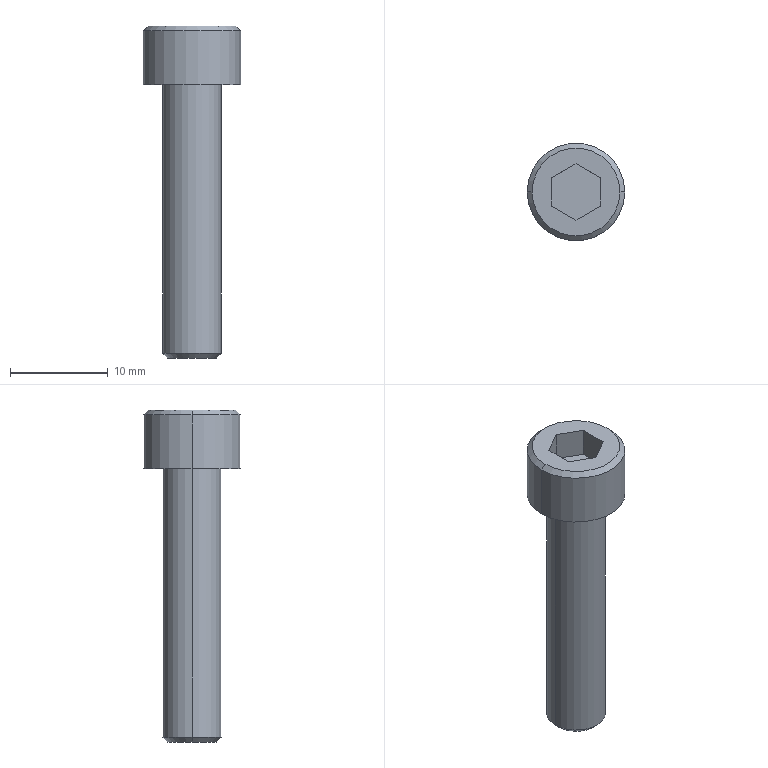Part | Creo | 1 solid | 18 faces | box 10 x 10 x 34 mm | volume 1192 mm3 | plane 10 | cone 4 | cylinder 4 | commonest cylinder face diameters 6 x2 10 x2
STEP:
#1=CARTESIAN_POINT('',(4.5,135.,-211.5));
#2=VERTEX_POINT('',#1);
#3=CARTESIAN_POINT('',(-4.5,135.,-211.5));
#4=VERTEX_POINT('',#3);
#5=CARTESIAN_POINT('',(0.,135.,-211.5));
#6=DIRECTION('',(0.,0.,1.));
#7=DIRECTION('',(1.,0.,0.));
#8=AXIS2_PLACEMENT_3D('',#5,#6,#7);
#9=CIRCLE('',#8,4.5);
#10=EDGE_CURVE('',#2,#4,#9,.T.);
#11=ORIENTED_EDGE('',*,*,#10,.F.);
#12=CARTESIAN_POINT('',(0.,135.,-211.5));
#13=DIRECTION('',(0.,0.,1.));
#14=DIRECTION('',(-1.,0.,0.));
#15=AXIS2_PLACEMENT_3D('',#12,#13,#14);
#16=CIRCLE('',#15,4.5);
#17=EDGE_CURVE('',#4,#2,#16,.T.);
#18=ORIENTED_EDGE('',*,*,#17,.F.);
#19=EDGE_LOOP('',(#11,#18));
#20=FACE_OUTER_BOUND('',#19,.F.);
#21=CARTESIAN_POINT('',(-2.5,133.557,-211.5));
#22=VERTEX_POINT('',#21);
#23=CARTESIAN_POINT('',(-2.5,136.443,-211.5));
#24=VERTEX_POINT('',#23);
#25=CARTESIAN_POINT('',(-2.5,133.557,-211.5));
#26=DIRECTION('',(0.,1.,0.));
#27=VECTOR('',#26,2.887);
#28=LINE('',#25,#27);
#29=EDGE_CURVE('',#22,#24,#28,.T.);
#30=ORIENTED_EDGE('',*,*,#29,.F.);
#31=CARTESIAN_POINT('',(0.,132.113,-211.5));
#32=VERTEX_POINT('',#31);
#33=CARTESIAN_POINT('',(0.,132.113,-211.5));
#34=DIRECTION('',(-0.866,0.5,0.));
#35=VECTOR('',#34,2.887);
#36=LINE('',#33,#35);
#37=EDGE_CURVE('',#32,#22,#36,.T.);
#38=ORIENTED_EDGE('',*,*,#37,.F.);
#39=CARTESIAN_POINT('',(2.5,133.557,-211.5));
#40=VERTEX_POINT('',#39);
#41=CARTESIAN_POINT('',(2.5,133.557,-211.5));
#42=DIRECTION('',(-0.866,-0.5,0.));
#43=VECTOR('',#42,2.887);
#44=LINE('',#41,#43);
#45=EDGE_CURVE('',#40,#32,#44,.T.);
#46=ORIENTED_EDGE('',*,*,#45,.F.);
#47=CARTESIAN_POINT('',(2.5,136.443,-211.5));
#48=VERTEX_POINT('',#47);
#49=CARTESIAN_POINT('',(2.5,136.443,-211.5));
#50=DIRECTION('',(0.,-1.,0.));
#51=VECTOR('',#50,2.887);
#52=LINE('',#49,#51);
#53=EDGE_CURVE('',#48,#40,#52,.T.);
#54=ORIENTED_EDGE('',*,*,#53,.F.);
#55=CARTESIAN_POINT('',(0.,137.887,-211.5));
#56=VERTEX_POINT('',#55);
#57=CARTESIAN_POINT('',(0.,137.887,-211.5));
#58=DIRECTION('',(0.866,-0.5,0.));
#59=VECTOR('',#58,2.887);
#60=LINE('',#57,#59);
#61=EDGE_CURVE('',#56,#48,#60,.T.);
#62=ORIENTED_EDGE('',*,*,#61,.F.);
#63=CARTESIAN_POINT('',(-2.5,136.443,-211.5));
#64=DIRECTION('',(0.866,0.5,0.));
#65=VECTOR('',#64,2.887);
#66=LINE('',#63,#65);
#67=EDGE_CURVE('',#24,#56,#66,.T.);
#68=ORIENTED_EDGE('',*,*,#67,.F.);
#69=EDGE_LOOP('',(#30,#38,#46,#54,#62,#68));
#70=FACE_BOUND('',#69,.F.);
#71=CARTESIAN_POINT('',(0.,135.,-211.5));
#72=DIRECTION('',(0.,0.,1.));
#73=DIRECTION('',(1.,0.,0.));
#74=AXIS2_PLACEMENT_3D('',#71,#72,#73);
#75=PLANE('',#74);
#76=ADVANCED_FACE('',(#20,#70),#75,.T.);
#77=ORIENTED_EDGE('',*,*,#10,.T.);
#78=CARTESIAN_POINT('',(-5.,135.,-212.));
#79=VERTEX_POINT('',#78);
#80=CARTESIAN_POINT('',(-4.5,135.,-211.5));
#81=DIRECTION('',(-0.7071,0.,-0.7071));
#82=VECTOR('',#81,0.7071);
#83=LINE('',#80,#82);
#84=EDGE_CURVE('',#4,#79,#83,.T.);
#85=ORIENTED_EDGE('',*,*,#84,.T.);
#86=CARTESIAN_POINT('',(5.,135.,-212.));
#87=VERTEX_POINT('',#86);
#88=CARTESIAN_POINT('',(0.,135.,-212.));
#89=DIRECTION('',(0.,0.,1.));
#90=DIRECTION('',(1.,0.,0.));
#91=AXIS2_PLACEMENT_3D('',#88,#89,#90);
#92=CIRCLE('',#91,5.);
#93=EDGE_CURVE('',#87,#79,#92,.T.);
#94=ORIENTED_EDGE('',*,*,#93,.F.);
#95=CARTESIAN_POINT('',(4.5,135.,-211.5));
#96=DIRECTION('',(0.7071,0.,-0.7071));
#97=VECTOR('',#96,0.7071);
#98=LINE('',#95,#97);
#99=EDGE_CURVE('',#2,#87,#98,.T.);
#100=ORIENTED_EDGE('',*,*,#99,.F.);
#101=EDGE_LOOP('',(#77,#85,#94,#100));
#102=FACE_OUTER_BOUND('',#101,.F.);
#103=CARTESIAN_POINT('',(0.,135.,-211.75));
#104=DIRECTION('',(0.,0.,-1.));
#105=DIRECTION('',(-1.,0.,0.));
#106=AXIS2_PLACEMENT_3D('',#103,#104,#105);
#107=CONICAL_SURFACE('',#106,4.75,45.);
#108=ADVANCED_FACE('',(#102),#107,.T.);
#109=ORIENTED_EDGE('',*,*,#17,.T.);
#110=ORIENTED_EDGE('',*,*,#99,.T.);
#111=CARTESIAN_POINT('',(0.,135.,-212.));
#112=DIRECTION('',(0.,0.,1.));
#113=DIRECTION('',(-1.,0.,0.));
#114=AXIS2_PLACEMENT_3D('',#111,#112,#113);
#115=CIRCLE('',#114,5.);
#116=EDGE_CURVE('',#79,#87,#115,.T.);
#117=ORIENTED_EDGE('',*,*,#116,.F.);
#118=ORIENTED_EDGE('',*,*,#84,.F.);
#119=EDGE_LOOP('',(#109,#110,#117,#118));
#120=FACE_OUTER_BOUND('',#119,.F.);
#121=CARTESIAN_POINT('',(0.,135.,-211.75));
#122=DIRECTION('',(0.,0.,-1.));
#123=DIRECTION('',(-1.,0.,0.));
#124=AXIS2_PLACEMENT_3D('',#121,#122,#123);
#125=CONICAL_SURFACE('',#124,4.75,45.);
#126=ADVANCED_FACE('',(#120),#125,.T.);
#127=ORIENTED_EDGE('',*,*,#116,.T.);
#128=CARTESIAN_POINT('',(5.,135.,-217.5));
#129=VERTEX_POINT('',#128);
#130=CARTESIAN_POINT('',(5.,135.,-217.5));
#131=DIRECTION('',(0.,0.,1.));
#132=VECTOR('',#131,5.5);
#133=LINE('',#130,#132);
#134=EDGE_CURVE('',#129,#87,#133,.T.);
#135=ORIENTED_EDGE('',*,*,#134,.F.);
#136=CARTESIAN_POINT('',(-5.,135.,-217.5));
#137=VERTEX_POINT('',#136);
#138=CARTESIAN_POINT('',(0.,135.,-217.5));
#139=DIRECTION('',(0.,0.,-1.));
#140=DIRECTION('',(1.,0.,0.));
#141=AXIS2_PLACEMENT_3D('',#138,#139,#140);
#142=CIRCLE('',#141,5.);
#143=EDGE_CURVE('',#129,#137,#142,.T.);
#144=ORIENTED_EDGE('',*,*,#143,.T.);
#145=CARTESIAN_POINT('',(-5.,135.,-217.5));
#146=DIRECTION('',(0.,0.,1.));
#147=VECTOR('',#146,5.5);
#148=LINE('',#145,#147);
#149=EDGE_CURVE('',#137,#79,#148,.T.);
#150=ORIENTED_EDGE('',*,*,#149,.T.);
#151=EDGE_LOOP('',(#127,#135,#144,#150));
#152=FACE_OUTER_BOUND('',#151,.F.);
#153=CARTESIAN_POINT('',(0.,135.,-217.5));
#154=DIRECTION('',(0.,0.,1.));
#155=DIRECTION('',(1.,0.,0.));
#156=AXIS2_PLACEMENT_3D('',#153,#154,#155);
#157=CYLINDRICAL_SURFACE('',#156,5.);
#158=ADVANCED_FACE('',(#152),#157,.T.);
#159=ORIENTED_EDGE('',*,*,#93,.T.);
#160=ORIENTED_EDGE('',*,*,#149,.F.);
#161=CARTESIAN_POINT('',(0.,135.,-217.5));
#162=DIRECTION('',(0.,0.,-1.));
#163=DIRECTION('',(-1.,0.,0.));
#164=AXIS2_PLACEMENT_3D('',#161,#162,#163);
#165=CIRCLE('',#164,5.);
#166=EDGE_CURVE('',#137,#129,#165,.T.);
#167=ORIENTED_EDGE('',*,*,#166,.T.);
#168=ORIENTED_EDGE('',*,*,#134,.T.);
#169=EDGE_LOOP('',(#159,#160,#167,#168));
#170=FACE_OUTER_BOUND('',#169,.F.);
#171=CARTESIAN_POINT('',(0.,135.,-217.5));
#172=DIRECTION('',(0.,0.,1.));
#173=DIRECTION('',(1.,0.,0.));
#174=AXIS2_PLACEMENT_3D('',#171,#172,#173);
#175=CYLINDRICAL_SURFACE('',#174,5.);
#176=ADVANCED_FACE('',(#170),#175,.T.);
#177=ORIENTED_EDGE('',*,*,#143,.F.);
#178=ORIENTED_EDGE('',*,*,#166,.F.);
#179=EDGE_LOOP('',(#177,#178));
#180=FACE_OUTER_BOUND('',#179,.F.);
#181=CARTESIAN_POINT('',(-3.,135.,-217.5));
#182=VERTEX_POINT('',#181);
#183=CARTESIAN_POINT('',(3.,135.,-217.5));
#184=VERTEX_POINT('',#183);
#185=CARTESIAN_POINT('',(0.,135.,-217.5));
#186=DIRECTION('',(0.,0.,1.));
#187=DIRECTION('',(-1.,0.,0.));
#188=AXIS2_PLACEMENT_3D('',#185,#186,#187);
#189=CIRCLE('',#188,3.);
#190=EDGE_CURVE('',#182,#184,#189,.T.);
#191=ORIENTED_EDGE('',*,*,#190,.F.);
#192=CARTESIAN_POINT('',(0.,135.,-217.5));
#193=DIRECTION('',(0.,0.,1.));
#194=DIRECTION('',(1.,0.,0.));
#195=AXIS2_PLACEMENT_3D('',#192,#193,#194);
#196=CIRCLE('',#195,3.);
#197=EDGE_CURVE('',#184,#182,#196,.T.);
#198=ORIENTED_EDGE('',*,*,#197,.F.);
#199=EDGE_LOOP('',(#191,#198));
#200=FACE_BOUND('',#199,.F.);
#201=CARTESIAN_POINT('',(0.,135.,-217.5));
#202=DIRECTION('',(0.,0.,-1.));
#203=DIRECTION('',(-1.,0.,0.));
#204=AXIS2_PLACEMENT_3D('',#201,#202,#203);
#205=PLANE('',#204);
#206=ADVANCED_FACE('',(#180,#200),#205,.T.);
#207=CARTESIAN_POINT('',(3.,135.,-245.));
#208=VERTEX_POINT('',#207);
#209=CARTESIAN_POINT('',(-3.,135.,-245.));
#210=VERTEX_POINT('',#209);
#211=CARTESIAN_POINT('',(0.,135.,-245.));
#212=DIRECTION('',(0.,0.,-1.));
#213=DIRECTION('',(1.,0.,0.));
#214=AXIS2_PLACEMENT_3D('',#211,#212,#213);
#215=CIRCLE('',#214,3.);
#216=EDGE_CURVE('',#208,#210,#215,.T.);
#217=ORIENTED_EDGE('',*,*,#216,.T.);
#218=CARTESIAN_POINT('',(-3.,135.,-217.5));
#219=DIRECTION('',(0.,0.,-1.));
#220=VECTOR('',#219,27.5);
#221=LINE('',#218,#220);
#222=EDGE_CURVE('',#182,#210,#221,.T.);
#223=ORIENTED_EDGE('',*,*,#222,.F.);
#224=ORIENTED_EDGE('',*,*,#190,.T.);
#225=CARTESIAN_POINT('',(3.,135.,-217.5));
#226=DIRECTION('',(0.,0.,-1.));
#227=VECTOR('',#226,27.5);
#228=LINE('',#225,#227);
#229=EDGE_CURVE('',#184,#208,#228,.T.);
#230=ORIENTED_EDGE('',*,*,#229,.T.);
#231=EDGE_LOOP('',(#217,#223,#224,#230));
#232=FACE_OUTER_BOUND('',#231,.F.);
#233=CARTESIAN_POINT('',(0.,135.,-217.5));
#234=DIRECTION('',(0.,0.,-1.));
#235=DIRECTION('',(-1.,0.,0.));
#236=AXIS2_PLACEMENT_3D('',#233,#234,#235);
#237=CYLINDRICAL_SURFACE('',#236,3.);
#238=ADVANCED_FACE('',(#232),#237,.T.);
#239=CARTESIAN_POINT('',(2.5,135.,-245.5));
#240=VERTEX_POINT('',#239);
#241=CARTESIAN_POINT('',(-2.5,135.,-245.5));
#242=VERTEX_POINT('',#241);
#243=CARTESIAN_POINT('',(0.,135.,-245.5));
#244=DIRECTION('',(0.,0.,-1.));
#245=DIRECTION('',(1.,0.,0.));
#246=AXIS2_PLACEMENT_3D('',#243,#244,#245);
#247=CIRCLE('',#246,2.5);
#248=EDGE_CURVE('',#240,#242,#247,.T.);
#249=ORIENTED_EDGE('',*,*,#248,.T.);
#250=CARTESIAN_POINT('',(-2.5,135.,-245.5));
#251=DIRECTION('',(-0.7071,0.,0.7071));
#252=VECTOR('',#251,0.7071);
#253=LINE('',#250,#252);
#254=EDGE_CURVE('',#242,#210,#253,.T.);
#255=ORIENTED_EDGE('',*,*,#254,.T.);
#256=ORIENTED_EDGE('',*,*,#216,.F.);
#257=CARTESIAN_POINT('',(2.5,135.,-245.5));
#258=DIRECTION('',(0.7071,0.,0.7071));
#259=VECTOR('',#258,0.7071);
#260=LINE('',#257,#259);
#261=EDGE_CURVE('',#240,#208,#260,.T.);
#262=ORIENTED_EDGE('',*,*,#261,.F.);
#263=EDGE_LOOP('',(#249,#255,#256,#262));
#264=FACE_OUTER_BOUND('',#263,.F.);
#265=CARTESIAN_POINT('',(0.,135.,-245.25));
#266=DIRECTION('',(0.,0.,1.));
#267=DIRECTION('',(1.,0.,0.));
#268=AXIS2_PLACEMENT_3D('',#265,#266,#267);
#269=CONICAL_SURFACE('',#268,2.75,45.);
#270=ADVANCED_FACE('',(#264),#269,.T.);
#271=CARTESIAN_POINT('',(0.,135.,-245.5));
#272=DIRECTION('',(0.,0.,-1.));
#273=DIRECTION('',(-1.,0.,0.));
#274=AXIS2_PLACEMENT_3D('',#271,#272,#273);
#275=CIRCLE('',#274,2.5);
#276=EDGE_CURVE('',#242,#240,#275,.T.);
#277=ORIENTED_EDGE('',*,*,#276,.F.);
#278=ORIENTED_EDGE('',*,*,#248,.F.);
#279=EDGE_LOOP('',(#277,#278));
#280=FACE_OUTER_BOUND('',#279,.F.);
#281=CARTESIAN_POINT('',(0.,135.,-245.5));
#282=DIRECTION('',(0.,0.,-1.));
#283=DIRECTION('',(-1.,0.,0.));
#284=AXIS2_PLACEMENT_3D('',#281,#282,#283);
#285=PLANE('',#284);
#286=ADVANCED_FACE('',(#280),#285,.T.);
#287=ORIENTED_EDGE('',*,*,#276,.T.);
#288=ORIENTED_EDGE('',*,*,#261,.T.);
#289=CARTESIAN_POINT('',(0.,135.,-245.));
#290=DIRECTION('',(0.,0.,-1.));
#291=DIRECTION('',(-1.,0.,0.));
#292=AXIS2_PLACEMENT_3D('',#289,#290,#291);
#293=CIRCLE('',#292,3.);
#294=EDGE_CURVE('',#210,#208,#293,.T.);
#295=ORIENTED_EDGE('',*,*,#294,.F.);
#296=ORIENTED_EDGE('',*,*,#254,.F.);
#297=EDGE_LOOP('',(#287,#288,#295,#296));
#298=FACE_OUTER_BOUND('',#297,.F.);
#299=CARTESIAN_POINT('',(0.,135.,-245.25));
#300=DIRECTION('',(0.,0.,1.));
#301=DIRECTION('',(1.,0.,0.));
#302=AXIS2_PLACEMENT_3D('',#299,#300,#301);
#303=CONICAL_SURFACE('',#302,2.75,45.);
#304=ADVANCED_FACE('',(#298),#303,.T.);
#305=ORIENTED_EDGE('',*,*,#294,.T.);
#306=ORIENTED_EDGE('',*,*,#229,.F.);
#307=ORIENTED_EDGE('',*,*,#197,.T.);
#308=ORIENTED_EDGE('',*,*,#222,.T.);
#309=EDGE_LOOP('',(#305,#306,#307,#308));
#310=FACE_OUTER_BOUND('',#309,.F.);
#311=CARTESIAN_POINT('',(0.,135.,-217.5));
#312=DIRECTION('',(0.,0.,-1.));
#313=DIRECTION('',(-1.,0.,0.));
#314=AXIS2_PLACEMENT_3D('',#311,#312,#313);
#315=CYLINDRICAL_SURFACE('',#314,3.);
#316=ADVANCED_FACE('',(#310),#315,.T.);
#317=ORIENTED_EDGE('',*,*,#29,.T.);
#318=CARTESIAN_POINT('',(-2.5,136.443,-214.5));
#319=VERTEX_POINT('',#318);
#320=CARTESIAN_POINT('',(-2.5,136.443,-211.5));
#321=DIRECTION('',(0.,0.,-1.));
#322=VECTOR('',#321,3.);
#323=LINE('',#320,#322);
#324=EDGE_CURVE('',#24,#319,#323,.T.);
#325=ORIENTED_EDGE('',*,*,#324,.T.);
#326=CARTESIAN_POINT('',(-2.5,133.557,-214.5));
#327=VERTEX_POINT('',#326);
#328=CARTESIAN_POINT('',(-2.5,133.557,-214.5));
#329=DIRECTION('',(0.,1.,0.));
#330=VECTOR('',#329,2.887);
#331=LINE('',#328,#330);
#332=EDGE_CURVE('',#327,#319,#331,.T.);
#333=ORIENTED_EDGE('',*,*,#332,.F.);
#334=CARTESIAN_POINT('',(-2.5,133.557,-211.5));
#335=DIRECTION('',(0.,0.,-1.));
#336=VECTOR('',#335,3.);
#337=LINE('',#334,#336);
#338=EDGE_CURVE('',#22,#327,#337,.T.);
#339=ORIENTED_EDGE('',*,*,#338,.F.);
#340=EDGE_LOOP('',(#317,#325,#333,#339));
#341=FACE_OUTER_BOUND('',#340,.F.);
#342=CARTESIAN_POINT('',(-2.5,135.,-213.));
#343=DIRECTION('',(-1.,0.,0.));
#344=DIRECTION('',(0.,0.,1.));
#345=AXIS2_PLACEMENT_3D('',#342,#343,#344);
#346=PLANE('',#345);
#347=ADVANCED_FACE('',(#341),#346,.F.);
#348=ORIENTED_EDGE('',*,*,#67,.T.);
#349=CARTESIAN_POINT('',(0.,137.887,-214.5));
#350=VERTEX_POINT('',#349);
#351=CARTESIAN_POINT('',(0.,137.887,-211.5));
#352=DIRECTION('',(0.,0.,-1.));
#353=VECTOR('',#352,3.);
#354=LINE('',#351,#353);
#355=EDGE_CURVE('',#56,#350,#354,.T.);
#356=ORIENTED_EDGE('',*,*,#355,.T.);
#357=CARTESIAN_POINT('',(0.,137.887,-214.5));
#358=DIRECTION('',(-0.866,-0.5,0.));
#359=VECTOR('',#358,2.887);
#360=LINE('',#357,#359);
#361=EDGE_CURVE('',#350,#319,#360,.T.);
#362=ORIENTED_EDGE('',*,*,#361,.T.);
#363=ORIENTED_EDGE('',*,*,#324,.F.);
#364=EDGE_LOOP('',(#348,#356,#362,#363));
#365=FACE_OUTER_BOUND('',#364,.F.);
#366=CARTESIAN_POINT('',(-1.25,137.165,-213.));
#367=DIRECTION('',(-0.5,0.866,0.));
#368=DIRECTION('',(-0.866,-0.5,0.));
#369=AXIS2_PLACEMENT_3D('',#366,#367,#368);
#370=PLANE('',#369);
#371=ADVANCED_FACE('',(#365),#370,.F.);
#372=ORIENTED_EDGE('',*,*,#61,.T.);
#373=CARTESIAN_POINT('',(2.5,136.443,-214.5));
#374=VERTEX_POINT('',#373);
#375=CARTESIAN_POINT('',(2.5,136.443,-211.5));
#376=DIRECTION('',(0.,0.,-1.));
#377=VECTOR('',#376,3.);
#378=LINE('',#375,#377);
#379=EDGE_CURVE('',#48,#374,#378,.T.);
#380=ORIENTED_EDGE('',*,*,#379,.T.);
#381=CARTESIAN_POINT('',(2.5,136.443,-214.5));
#382=DIRECTION('',(-0.866,0.5,0.));
#383=VECTOR('',#382,2.887);
#384=LINE('',#381,#383);
#385=EDGE_CURVE('',#374,#350,#384,.T.);
#386=ORIENTED_EDGE('',*,*,#385,.T.);
#387=ORIENTED_EDGE('',*,*,#355,.F.);
#388=EDGE_LOOP('',(#372,#380,#386,#387));
#389=FACE_OUTER_BOUND('',#388,.F.);
#390=CARTESIAN_POINT('',(1.25,137.165,-213.));
#391=DIRECTION('',(0.5,0.866,0.));
#392=DIRECTION('',(-0.866,0.5,0.));
#393=AXIS2_PLACEMENT_3D('',#390,#391,#392);
#394=PLANE('',#393);
#395=ADVANCED_FACE('',(#389),#394,.F.);
#396=ORIENTED_EDGE('',*,*,#53,.T.);
#397=CARTESIAN_POINT('',(2.5,133.557,-214.5));
#398=VERTEX_POINT('',#397);
#399=CARTESIAN_POINT('',(2.5,133.557,-211.5));
#400=DIRECTION('',(0.,0.,-1.));
#401=VECTOR('',#400,3.);
#402=LINE('',#399,#401);
#403=EDGE_CURVE('',#40,#398,#402,.T.);
#404=ORIENTED_EDGE('',*,*,#403,.T.);
#405=CARTESIAN_POINT('',(2.5,136.443,-214.5));
#406=DIRECTION('',(0.,-1.,0.));
#407=VECTOR('',#406,2.887);
#408=LINE('',#405,#407);
#409=EDGE_CURVE('',#374,#398,#408,.T.);
#410=ORIENTED_EDGE('',*,*,#409,.F.);
#411=ORIENTED_EDGE('',*,*,#379,.F.);
#412=EDGE_LOOP('',(#396,#404,#410,#411));
#413=FACE_OUTER_BOUND('',#412,.F.);
#414=CARTESIAN_POINT('',(2.5,135.,-213.));
#415=DIRECTION('',(1.,0.,0.));
#416=DIRECTION('',(0.,0.,-1.));
#417=AXIS2_PLACEMENT_3D('',#414,#415,#416);
#418=PLANE('',#417);
#419=ADVANCED_FACE('',(#413),#418,.F.);
#420=ORIENTED_EDGE('',*,*,#45,.T.);
#421=CARTESIAN_POINT('',(0.,132.113,-214.5));
#422=VERTEX_POINT('',#421);
#423=CARTESIAN_POINT('',(0.,132.113,-211.5));
#424=DIRECTION('',(0.,0.,-1.));
#425=VECTOR('',#424,3.);
#426=LINE('',#423,#425);
#427=EDGE_CURVE('',#32,#422,#426,.T.);
#428=ORIENTED_EDGE('',*,*,#427,.T.);
#429=CARTESIAN_POINT('',(0.,132.113,-214.5));
#430=DIRECTION('',(0.866,0.5,0.));
#431=VECTOR('',#430,2.887);
#432=LINE('',#429,#431);
#433=EDGE_CURVE('',#422,#398,#432,.T.);
#434=ORIENTED_EDGE('',*,*,#433,.T.);
#435=ORIENTED_EDGE('',*,*,#403,.F.);
#436=EDGE_LOOP('',(#420,#428,#434,#435));
#437=FACE_OUTER_BOUND('',#436,.F.);
#438=CARTESIAN_POINT('',(1.25,132.835,-213.));
#439=DIRECTION('',(0.5,-0.866,0.));
#440=DIRECTION('',(0.866,0.5,0.));
#441=AXIS2_PLACEMENT_3D('',#438,#439,#440);
#442=PLANE('',#441);
#443=ADVANCED_FACE('',(#437),#442,.F.);
#444=ORIENTED_EDGE('',*,*,#37,.T.);
#445=ORIENTED_EDGE('',*,*,#338,.T.);
#446=CARTESIAN_POINT('',(-2.5,133.557,-214.5));
#447=DIRECTION('',(0.866,-0.5,0.));
#448=VECTOR('',#447,2.887);
#449=LINE('',#446,#448);
#450=EDGE_CURVE('',#327,#422,#449,.T.);
#451=ORIENTED_EDGE('',*,*,#450,.T.);
#452=ORIENTED_EDGE('',*,*,#427,.F.);
#453=EDGE_LOOP('',(#444,#445,#451,#452));
#454=FACE_OUTER_BOUND('',#453,.F.);
#455=CARTESIAN_POINT('',(-1.25,132.835,-213.));
#456=DIRECTION('',(-0.5,-0.866,0.));
#457=DIRECTION('',(0.866,-0.5,0.));
#458=AXIS2_PLACEMENT_3D('',#455,#456,#457);
#459=PLANE('',#458);
#460=ADVANCED_FACE('',(#454),#459,.F.);
#461=ORIENTED_EDGE('',*,*,#433,.F.);
#462=ORIENTED_EDGE('',*,*,#450,.F.);
#463=ORIENTED_EDGE('',*,*,#332,.T.);
#464=ORIENTED_EDGE('',*,*,#361,.F.);
#465=ORIENTED_EDGE('',*,*,#385,.F.);
#466=ORIENTED_EDGE('',*,*,#409,.T.);
#467=EDGE_LOOP('',(#461,#462,#463,#464,#465,#466));
#468=FACE_OUTER_BOUND('',#467,.F.);
#469=CARTESIAN_POINT('',(0.,135.,-214.5));
#470=DIRECTION('',(0.,0.,-1.));
#471=DIRECTION('',(-1.,0.,0.));
#472=AXIS2_PLACEMENT_3D('',#469,#470,#471);
#473=PLANE('',#472);
#474=ADVANCED_FACE('',(#468),#473,.F.);
#475=CLOSED_SHELL('',(#76,#108,#126,#158,#176,#206,#238,#270,#286,#304,#316,#347,#371,#395,#419,#443,#460,#474));
#476=MANIFOLD_SOLID_BREP('',#475);
#477=(LENGTH_UNIT()NAMED_UNIT(*)SI_UNIT(.MILLI.,.METRE.));
#478=UNCERTAINTY_MEASURE_WITH_UNIT(LENGTH_MEASURE(0.003682),#477,'','');
#479=(NAMED_UNIT(*)PLANE_ANGLE_UNIT()SI_UNIT($,.RADIAN.));
#480=PLANE_ANGLE_MEASURE_WITH_UNIT(PLANE_ANGLE_MEASURE(0.01745),#479);
#481=(CONVERSION_BASED_UNIT('DEGREE',#480)NAMED_UNIT(*)PLANE_ANGLE_UNIT());
#482=(NAMED_UNIT(*)SI_UNIT($,.STERADIAN.)SOLID_ANGLE_UNIT());
#483=(GEOMETRIC_REPRESENTATION_CONTEXT(3)GLOBAL_UNCERTAINTY_ASSIGNED_CONTEXT((#478))GLOBAL_UNIT_ASSIGNED_CONTEXT((#477,#481,#482))REPRESENTATION_CONTEXT('',''));
#484=ADVANCED_BREP_SHAPE_REPRESENTATION('',(#476),#483);